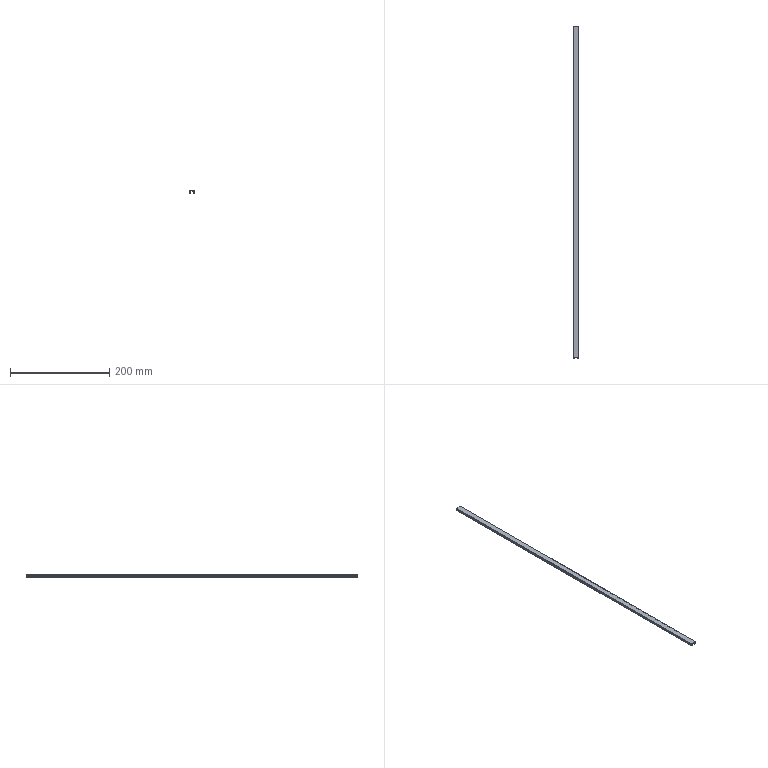Part | STEP file | DEWALT-DWE7492-B22 | 1 solid | 24 faces | box 11.9 x 670 x 4.7 mm | volume 19402 mm3 | plane 18 | cylinder 6 | commonest cylinder face diameters 1 x6